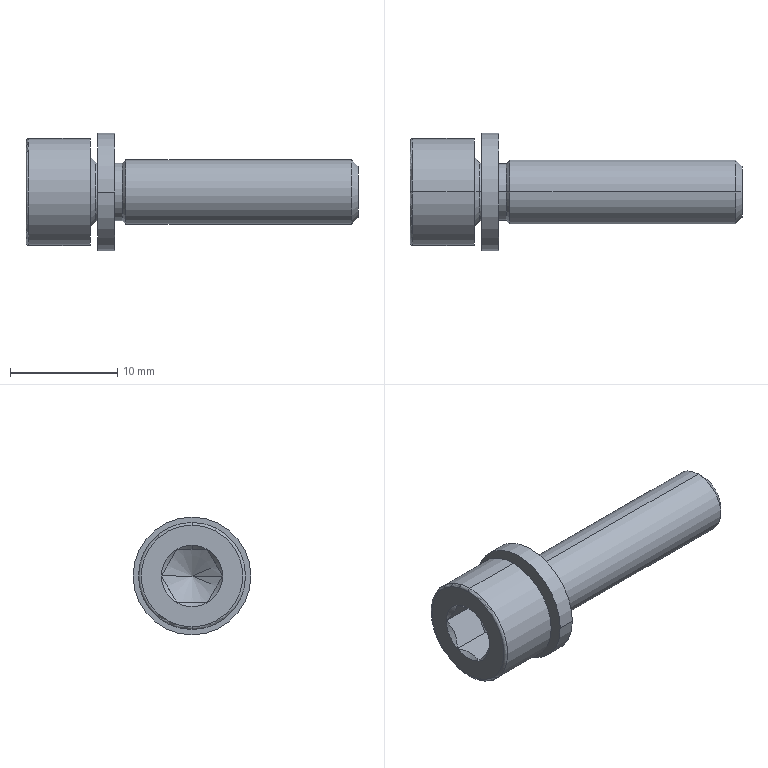Part | SolidWorks | features RevCut 2, Revolution 2, Chamfer 1, Cut 1, Fillet 1 | 2 solids | 48 faces | box 31 x 11 x 11 mm | volume 1178 mm3 | plane 17 | cone 15 | cylinder 10 | torus 6 | commonest cylinder face diameters 5.35 x2 5.62 x2 6 x2 10 x2 11 x2
STEP:
#1=CARTESIAN_POINT('',(8.28,-5.5,0.));
#2=VERTEX_POINT('',#1);
#3=CARTESIAN_POINT('',(8.28,5.5,0.));
#4=VERTEX_POINT('',#3);
#5=CARTESIAN_POINT('',(8.28,0.,0.));
#6=DIRECTION('',(-1.,0.,0.));
#7=DIRECTION('',(0.,-1.,0.));
#8=AXIS2_PLACEMENT_3D('',#5,#6,#7);
#9=CIRCLE('',#8,5.5);
#10=EDGE_CURVE('',#2,#4,#9,.T.);
#11=ORIENTED_EDGE('',*,*,#10,.T.);
#12=CARTESIAN_POINT('',(6.68,5.5,0.));
#13=VERTEX_POINT('',#12);
#14=CARTESIAN_POINT('',(0.,5.5,0.));
#15=DIRECTION('',(-1.,0.,0.));
#16=VECTOR('',#15,1000.);
#17=LINE('',#14,#16);
#18=EDGE_CURVE('',#4,#13,#17,.T.);
#19=ORIENTED_EDGE('',*,*,#18,.T.);
#20=CARTESIAN_POINT('',(6.68,-5.5,0.));
#21=VERTEX_POINT('',#20);
#22=CARTESIAN_POINT('',(6.68,0.,0.));
#23=DIRECTION('',(-1.,0.,0.));
#24=DIRECTION('',(0.,-1.,0.));
#25=AXIS2_PLACEMENT_3D('',#22,#23,#24);
#26=CIRCLE('',#25,5.5);
#27=EDGE_CURVE('',#21,#13,#26,.T.);
#28=ORIENTED_EDGE('',*,*,#27,.F.);
#29=CARTESIAN_POINT('',(0.,-5.5,0.));
#30=DIRECTION('',(-1.,0.,0.));
#31=VECTOR('',#30,1000.);
#32=LINE('',#29,#31);
#33=EDGE_CURVE('',#2,#21,#32,.T.);
#34=ORIENTED_EDGE('',*,*,#33,.F.);
#35=EDGE_LOOP('',(#11,#19,#28,#34));
#36=FACE_OUTER_BOUND('',#35,.T.);
#37=CARTESIAN_POINT('',(0.,0.,0.));
#38=DIRECTION('',(-1.,0.,0.));
#39=DIRECTION('',(0.,-1.,0.));
#40=AXIS2_PLACEMENT_3D('',#37,#38,#39);
#41=CYLINDRICAL_SURFACE('',#40,5.5);
#42=ADVANCED_FACE('',(#36),#41,.T.);
#43=CARTESIAN_POINT('',(8.28,2.81,0.));
#44=VERTEX_POINT('',#43);
#45=CARTESIAN_POINT('',(8.28,-2.81,0.));
#46=VERTEX_POINT('',#45);
#47=CARTESIAN_POINT('',(8.28,0.,0.));
#48=DIRECTION('',(-1.,0.,0.));
#49=DIRECTION('',(0.,-1.,0.));
#50=AXIS2_PLACEMENT_3D('',#47,#48,#49);
#51=CIRCLE('',#50,2.81);
#52=EDGE_CURVE('',#44,#46,#51,.T.);
#53=ORIENTED_EDGE('',*,*,#52,.F.);
#54=CARTESIAN_POINT('',(6.68,2.81,0.));
#55=VERTEX_POINT('',#54);
#56=CARTESIAN_POINT('',(0.,2.81,0.));
#57=DIRECTION('',(-1.,0.,0.));
#58=VECTOR('',#57,1000.);
#59=LINE('',#56,#58);
#60=EDGE_CURVE('',#44,#55,#59,.T.);
#61=ORIENTED_EDGE('',*,*,#60,.T.);
#62=CARTESIAN_POINT('',(6.68,-2.81,0.));
#63=VERTEX_POINT('',#62);
#64=CARTESIAN_POINT('',(6.68,0.,0.));
#65=DIRECTION('',(-1.,0.,0.));
#66=DIRECTION('',(0.,-1.,0.));
#67=AXIS2_PLACEMENT_3D('',#64,#65,#66);
#68=CIRCLE('',#67,2.81);
#69=EDGE_CURVE('',#55,#63,#68,.T.);
#70=ORIENTED_EDGE('',*,*,#69,.T.);
#71=CARTESIAN_POINT('',(0.,-2.81,0.));
#72=DIRECTION('',(-1.,0.,0.));
#73=VECTOR('',#72,1000.);
#74=LINE('',#71,#73);
#75=EDGE_CURVE('',#46,#63,#74,.T.);
#76=ORIENTED_EDGE('',*,*,#75,.F.);
#77=EDGE_LOOP('',(#53,#61,#70,#76));
#78=FACE_OUTER_BOUND('',#77,.T.);
#79=CARTESIAN_POINT('',(0.,0.,0.));
#80=DIRECTION('',(-1.,0.,0.));
#81=DIRECTION('',(0.,-1.,0.));
#82=AXIS2_PLACEMENT_3D('',#79,#80,#81);
#83=CYLINDRICAL_SURFACE('',#82,2.81);
#84=ADVANCED_FACE('',(#78),#83,.F.);
#85=ORIENTED_EDGE('',*,*,#60,.F.);
#86=CARTESIAN_POINT('',(8.28,0.,0.));
#87=DIRECTION('',(-1.,0.,0.));
#88=DIRECTION('',(0.,-1.,0.));
#89=AXIS2_PLACEMENT_3D('',#86,#87,#88);
#90=CIRCLE('',#89,2.81);
#91=EDGE_CURVE('',#46,#44,#90,.T.);
#92=ORIENTED_EDGE('',*,*,#91,.F.);
#93=ORIENTED_EDGE('',*,*,#75,.T.);
#94=CARTESIAN_POINT('',(6.68,0.,0.));
#95=DIRECTION('',(-1.,0.,0.));
#96=DIRECTION('',(0.,-1.,0.));
#97=AXIS2_PLACEMENT_3D('',#94,#95,#96);
#98=CIRCLE('',#97,2.81);
#99=EDGE_CURVE('',#63,#55,#98,.T.);
#100=ORIENTED_EDGE('',*,*,#99,.T.);
#101=EDGE_LOOP('',(#85,#92,#93,#100));
#102=FACE_OUTER_BOUND('',#101,.T.);
#103=CARTESIAN_POINT('',(0.,0.,0.));
#104=DIRECTION('',(-1.,0.,0.));
#105=DIRECTION('',(0.,-1.,0.));
#106=AXIS2_PLACEMENT_3D('',#103,#104,#105);
#107=CYLINDRICAL_SURFACE('',#106,2.81);
#108=ADVANCED_FACE('',(#102),#107,.F.);
#109=ORIENTED_EDGE('',*,*,#99,.F.);
#110=ORIENTED_EDGE('',*,*,#69,.F.);
#111=EDGE_LOOP('',(#109,#110));
#112=FACE_BOUND('',#111,.T.);
#113=ORIENTED_EDGE('',*,*,#27,.T.);
#114=CARTESIAN_POINT('',(6.68,0.,0.));
#115=DIRECTION('',(-1.,0.,0.));
#116=DIRECTION('',(0.,-1.,0.));
#117=AXIS2_PLACEMENT_3D('',#114,#115,#116);
#118=CIRCLE('',#117,5.5);
#119=EDGE_CURVE('',#13,#21,#118,.T.);
#120=ORIENTED_EDGE('',*,*,#119,.T.);
#121=EDGE_LOOP('',(#113,#120));
#122=FACE_OUTER_BOUND('',#121,.T.);
#123=CARTESIAN_POINT('',(6.68,-2.81,0.));
#124=DIRECTION('',(1.,0.,0.));
#125=DIRECTION('',(0.,1.,0.));
#126=AXIS2_PLACEMENT_3D('',#123,#124,#125);
#127=PLANE('',#126);
#128=ADVANCED_FACE('',(#112,#122),#127,.F.);
#129=ORIENTED_EDGE('',*,*,#18,.F.);
#130=CARTESIAN_POINT('',(8.28,0.,0.));
#131=DIRECTION('',(-1.,0.,0.));
#132=DIRECTION('',(0.,-1.,0.));
#133=AXIS2_PLACEMENT_3D('',#130,#131,#132);
#134=CIRCLE('',#133,5.5);
#135=EDGE_CURVE('',#4,#2,#134,.T.);
#136=ORIENTED_EDGE('',*,*,#135,.T.);
#137=ORIENTED_EDGE('',*,*,#33,.T.);
#138=ORIENTED_EDGE('',*,*,#119,.F.);
#139=EDGE_LOOP('',(#129,#136,#137,#138));
#140=FACE_OUTER_BOUND('',#139,.T.);
#141=CARTESIAN_POINT('',(0.,0.,0.));
#142=DIRECTION('',(-1.,0.,0.));
#143=DIRECTION('',(0.,-1.,0.));
#144=AXIS2_PLACEMENT_3D('',#141,#142,#143);
#145=CYLINDRICAL_SURFACE('',#144,5.5);
#146=ADVANCED_FACE('',(#140),#145,.T.);
#147=ORIENTED_EDGE('',*,*,#10,.F.);
#148=ORIENTED_EDGE('',*,*,#135,.F.);
#149=EDGE_LOOP('',(#147,#148));
#150=FACE_OUTER_BOUND('',#149,.T.);
#151=ORIENTED_EDGE('',*,*,#91,.T.);
#152=ORIENTED_EDGE('',*,*,#52,.T.);
#153=EDGE_LOOP('',(#151,#152));
#154=FACE_BOUND('',#153,.T.);
#155=CARTESIAN_POINT('',(8.28,-5.5,0.));
#156=DIRECTION('',(-1.,0.,0.));
#157=DIRECTION('',(0.,-1.,0.));
#158=AXIS2_PLACEMENT_3D('',#155,#156,#157);
#159=PLANE('',#158);
#160=ADVANCED_FACE('',(#150,#154),#159,.F.);
#161=CLOSED_SHELL('',(#42,#84,#108,#128,#146,#160));
#162=MANIFOLD_SOLID_BREP('',#161);
#163=CARTESIAN_POINT('',(31.,0.,-2.4));
#164=VERTEX_POINT('',#163);
#165=CARTESIAN_POINT('',(31.,0.,2.4));
#166=VERTEX_POINT('',#165);
#167=CARTESIAN_POINT('',(31.,0.,0.));
#168=DIRECTION('',(1.,0.,0.));
#169=DIRECTION('',(0.,0.,-1.));
#170=AXIS2_PLACEMENT_3D('',#167,#168,#169);
#171=CIRCLE('',#170,2.4);
#172=EDGE_CURVE('',#164,#166,#171,.T.);
#173=ORIENTED_EDGE('',*,*,#172,.F.);
#174=CARTESIAN_POINT('',(30.4,0.,-3.));
#175=VERTEX_POINT('',#174);
#176=CARTESIAN_POINT('',(31.,0.,-2.4));
#177=DIRECTION('',(-0.7071,0.,-0.7071));
#178=VECTOR('',#177,1000.);
#179=LINE('',#176,#178);
#180=EDGE_CURVE('',#164,#175,#179,.T.);
#181=ORIENTED_EDGE('',*,*,#180,.T.);
#182=CARTESIAN_POINT('',(30.4,0.,3.));
#183=VERTEX_POINT('',#182);
#184=CARTESIAN_POINT('',(30.4,0.,0.));
#185=DIRECTION('',(-1.,0.,0.));
#186=DIRECTION('',(0.,0.,-1.));
#187=AXIS2_PLACEMENT_3D('',#184,#185,#186);
#188=CIRCLE('',#187,3.);
#189=EDGE_CURVE('',#183,#175,#188,.T.);
#190=ORIENTED_EDGE('',*,*,#189,.F.);
#191=CARTESIAN_POINT('',(31.,0.,2.4));
#192=DIRECTION('',(-0.7071,0.,0.7071));
#193=VECTOR('',#192,1000.);
#194=LINE('',#191,#193);
#195=EDGE_CURVE('',#166,#183,#194,.T.);
#196=ORIENTED_EDGE('',*,*,#195,.F.);
#197=EDGE_LOOP('',(#173,#181,#190,#196));
#198=FACE_OUTER_BOUND('',#197,.T.);
#199=CARTESIAN_POINT('',(31.,0.,0.));
#200=DIRECTION('',(-1.,0.,0.));
#201=DIRECTION('',(0.,0.,1.));
#202=AXIS2_PLACEMENT_3D('',#199,#200,#201);
#203=CONICAL_SURFACE('',#202,2.4,0.7854);
#204=ADVANCED_FACE('',(#198),#203,.T.);
#205=CARTESIAN_POINT('',(0.25,0.,-5.));
#206=VERTEX_POINT('',#205);
#207=CARTESIAN_POINT('',(0.25,0.,5.));
#208=VERTEX_POINT('',#207);
#209=CARTESIAN_POINT('',(0.25,0.,0.));
#210=DIRECTION('',(1.,0.,0.));
#211=DIRECTION('',(0.,0.,1.));
#212=AXIS2_PLACEMENT_3D('',#209,#210,#211);
#213=CIRCLE('',#212,5.);
#214=EDGE_CURVE('',#206,#208,#213,.T.);
#215=ORIENTED_EDGE('',*,*,#214,.F.);
#216=CARTESIAN_POINT('',(0.,0.,-4.75));
#217=VERTEX_POINT('',#216);
#218=CARTESIAN_POINT('',(0.25,0.,-4.75));
#219=DIRECTION('',(0.,1.,0.));
#220=DIRECTION('',(0.,0.,1.));
#221=AXIS2_PLACEMENT_3D('',#218,#219,#220);
#222=CIRCLE('',#221,0.25);
#223=EDGE_CURVE('',#206,#217,#222,.T.);
#224=ORIENTED_EDGE('',*,*,#223,.T.);
#225=CARTESIAN_POINT('',(0.,0.,4.75));
#226=VERTEX_POINT('',#225);
#227=CARTESIAN_POINT('',(0.,0.,0.));
#228=DIRECTION('',(-1.,0.,0.));
#229=DIRECTION('',(0.,0.,1.));
#230=AXIS2_PLACEMENT_3D('',#227,#228,#229);
#231=CIRCLE('',#230,4.75);
#232=EDGE_CURVE('',#226,#217,#231,.T.);
#233=ORIENTED_EDGE('',*,*,#232,.F.);
#234=CARTESIAN_POINT('',(0.25,0.,4.75));
#235=DIRECTION('',(0.,-1.,0.));
#236=DIRECTION('',(0.,0.,-1.));
#237=AXIS2_PLACEMENT_3D('',#234,#235,#236);
#238=CIRCLE('',#237,0.25);
#239=EDGE_CURVE('',#208,#226,#238,.T.);
#240=ORIENTED_EDGE('',*,*,#239,.F.);
#241=EDGE_LOOP('',(#215,#224,#233,#240));
#242=FACE_OUTER_BOUND('',#241,.T.);
#243=CARTESIAN_POINT('',(0.25,0.,0.));
#244=DIRECTION('',(-1.,0.,0.));
#245=DIRECTION('',(0.,0.,1.));
#246=AXIS2_PLACEMENT_3D('',#243,#244,#245);
#247=TOROIDAL_SURFACE('',#246,4.75,0.25);
#248=ADVANCED_FACE('',(#242),#247,.T.);
#249=CARTESIAN_POINT('',(5.351,0.,0.));
#250=VERTEX_POINT('',#249);
#251=CARTESIAN_POINT('',(3.7,-2.86,0.));
#252=VERTEX_POINT('',#251);
#253=CARTESIAN_POINT('',(5.351,0.,0.));
#254=DIRECTION('',(-0.5,-0.866,0.));
#255=VECTOR('',#254,1000.);
#256=LINE('',#253,#255);
#257=EDGE_CURVE('',#250,#252,#256,.T.);
#258=ORIENTED_EDGE('',*,*,#257,.F.);
#259=CARTESIAN_POINT('',(3.7,2.86,0.));
#260=VERTEX_POINT('',#259);
#261=CARTESIAN_POINT('',(5.351,0.,0.));
#262=DIRECTION('',(-0.5,0.866,0.));
#263=VECTOR('',#262,1000.);
#264=LINE('',#261,#263);
#265=EDGE_CURVE('',#250,#260,#264,.T.);
#266=ORIENTED_EDGE('',*,*,#265,.T.);
#267=CARTESIAN_POINT('',(3.7,1.43,-2.477));
#268=VERTEX_POINT('',#267);
#269=CARTESIAN_POINT('',(3.7,0.,0.));
#270=DIRECTION('',(-1.,0.,0.));
#271=DIRECTION('',(0.,-1.,0.));
#272=AXIS2_PLACEMENT_3D('',#269,#270,#271);
#273=CIRCLE('',#272,2.86);
#274=EDGE_CURVE('',#260,#268,#273,.T.);
#275=ORIENTED_EDGE('',*,*,#274,.T.);
#276=CARTESIAN_POINT('',(3.7,-1.43,-2.477));
#277=VERTEX_POINT('',#276);
#278=CARTESIAN_POINT('',(3.7,0.,0.));
#279=DIRECTION('',(-1.,0.,0.));
#280=DIRECTION('',(0.,-1.,0.));
#281=AXIS2_PLACEMENT_3D('',#278,#279,#280);
#282=CIRCLE('',#281,2.86);
#283=EDGE_CURVE('',#268,#277,#282,.T.);
#284=ORIENTED_EDGE('',*,*,#283,.T.);
#285=CARTESIAN_POINT('',(3.7,0.,0.));
#286=DIRECTION('',(-1.,0.,0.));
#287=DIRECTION('',(0.,-1.,0.));
#288=AXIS2_PLACEMENT_3D('',#285,#286,#287);
#289=CIRCLE('',#288,2.86);
#290=EDGE_CURVE('',#277,#252,#289,.T.);
#291=ORIENTED_EDGE('',*,*,#290,.T.);
#292=EDGE_LOOP('',(#258,#266,#275,#284,#291));
#293=FACE_OUTER_BOUND('',#292,.T.);
#294=CARTESIAN_POINT('',(-994.649,0.,0.));
#295=DIRECTION('',(-1.,0.,0.));
#296=DIRECTION('',(0.,-1.,0.));
#297=AXIS2_PLACEMENT_3D('',#294,#295,#296);
#298=CONICAL_SURFACE('',#297,1732.051,1.047);
#299=ADVANCED_FACE('',(#293),#298,.F.);
#300=CARTESIAN_POINT('',(0.3832,0.,2.477));
#301=VERTEX_POINT('',#300);
#302=CARTESIAN_POINT('',(0.,1.43,2.477));
#303=VERTEX_POINT('',#302);
#304=CARTESIAN_POINT('',(0.3832,0.,2.477));
#305=CARTESIAN_POINT('',(0.3832,0.2515,2.477));
#306=CARTESIAN_POINT('',(0.3444,0.4963,2.477));
#307=CARTESIAN_POINT('',(0.2078,0.9759,2.477));
#308=CARTESIAN_POINT('',(0.1107,1.209,2.477));
#309=CARTESIAN_POINT('',(0.,1.43,2.477));
#310=B_SPLINE_CURVE_WITH_KNOTS('',3,(#304,#305,#306,#307,#308,#309),.UNSPECIFIED.,.F.,.F.,(4,2,4),(0.003339,0.004081,0.004823),.UNSPECIFIED.);
#311=EDGE_CURVE('',#301,#303,#310,.T.);
#312=ORIENTED_EDGE('',*,*,#311,.F.);
#313=CARTESIAN_POINT('',(0.,0.,2.86));
#314=VERTEX_POINT('',#313);
#315=CARTESIAN_POINT('',(0.3832,0.,2.477));
#316=DIRECTION('',(-0.7071,0.,0.7071));
#317=VECTOR('',#316,1000.);
#318=LINE('',#315,#317);
#319=EDGE_CURVE('',#301,#314,#318,.T.);
#320=ORIENTED_EDGE('',*,*,#319,.T.);
#321=CARTESIAN_POINT('',(0.,0.,0.));
#322=DIRECTION('',(1.,0.,0.));
#323=DIRECTION('',(0.,0.,-1.));
#324=AXIS2_PLACEMENT_3D('',#321,#322,#323);
#325=CIRCLE('',#324,2.86);
#326=EDGE_CURVE('',#303,#314,#325,.T.);
#327=ORIENTED_EDGE('',*,*,#326,.F.);
#328=EDGE_LOOP('',(#312,#320,#327));
#329=FACE_OUTER_BOUND('',#328,.T.);
#330=CARTESIAN_POINT('',(0.3832,0.,0.));
#331=DIRECTION('',(-1.,0.,0.));
#332=DIRECTION('',(0.,0.,1.));
#333=AXIS2_PLACEMENT_3D('',#330,#331,#332);
#334=CONICAL_SURFACE('',#333,2.477,0.7854);
#335=ADVANCED_FACE('',(#329),#334,.F.);
#336=CARTESIAN_POINT('',(9.325,0.,-3.));
#337=VERTEX_POINT('',#336);
#338=CARTESIAN_POINT('',(9.325,0.,3.));
#339=VERTEX_POINT('',#338);
#340=CARTESIAN_POINT('',(9.325,0.,0.));
#341=DIRECTION('',(1.,0.,0.));
#342=DIRECTION('',(0.,0.,-1.));
#343=AXIS2_PLACEMENT_3D('',#340,#341,#342);
#344=CIRCLE('',#343,3.);
#345=EDGE_CURVE('',#337,#339,#344,.T.);
#346=ORIENTED_EDGE('',*,*,#345,.T.);
#347=CARTESIAN_POINT('',(0.,0.,3.));
#348=DIRECTION('',(1.,0.,0.));
#349=VECTOR('',#348,1000.);
#350=LINE('',#347,#349);
#351=EDGE_CURVE('',#339,#183,#350,.T.);
#352=ORIENTED_EDGE('',*,*,#351,.T.);
#353=ORIENTED_EDGE('',*,*,#189,.T.);
#354=CARTESIAN_POINT('',(0.,0.,-3.));
#355=DIRECTION('',(1.,0.,0.));
#356=VECTOR('',#355,1000.);
#357=LINE('',#354,#356);
#358=EDGE_CURVE('',#337,#175,#357,.T.);
#359=ORIENTED_EDGE('',*,*,#358,.F.);
#360=EDGE_LOOP('',(#346,#352,#353,#359));
#361=FACE_OUTER_BOUND('',#360,.T.);
#362=CARTESIAN_POINT('',(0.,0.,0.));
#363=DIRECTION('',(1.,0.,0.));
#364=DIRECTION('',(0.,0.,-1.));
#365=AXIS2_PLACEMENT_3D('',#362,#363,#364);
#366=CYLINDRICAL_SURFACE('',#365,3.);
#367=ADVANCED_FACE('',(#361),#366,.T.);
#368=CARTESIAN_POINT('',(9.,0.,-2.675));
#369=VERTEX_POINT('',#368);
#370=CARTESIAN_POINT('',(9.,0.,2.675));
#371=VERTEX_POINT('',#370);
#372=CARTESIAN_POINT('',(9.,0.,0.));
#373=DIRECTION('',(1.,0.,0.));
#374=DIRECTION('',(0.,0.,-1.));
#375=AXIS2_PLACEMENT_3D('',#372,#373,#374);
#376=CIRCLE('',#375,2.675);
#377=EDGE_CURVE('',#369,#371,#376,.T.);
#378=ORIENTED_EDGE('',*,*,#377,.T.);
#379=CARTESIAN_POINT('',(9.325,0.,3.));
#380=DIRECTION('',(0.7071,0.,0.7071));
#381=VECTOR('',#380,1000.);
#382=LINE('',#379,#381);
#383=EDGE_CURVE('',#371,#339,#382,.T.);
#384=ORIENTED_EDGE('',*,*,#383,.T.);
#385=ORIENTED_EDGE('',*,*,#345,.F.);
#386=CARTESIAN_POINT('',(9.325,0.,-3.));
#387=DIRECTION('',(0.7071,0.,-0.7071));
#388=VECTOR('',#387,1000.);
#389=LINE('',#386,#388);
#390=EDGE_CURVE('',#369,#337,#389,.T.);
#391=ORIENTED_EDGE('',*,*,#390,.F.);
#392=EDGE_LOOP('',(#378,#384,#385,#391));
#393=FACE_OUTER_BOUND('',#392,.T.);
#394=CARTESIAN_POINT('',(9.325,0.,0.));
#395=DIRECTION('',(1.,0.,0.));
#396=DIRECTION('',(0.,0.,-1.));
#397=AXIS2_PLACEMENT_3D('',#394,#395,#396);
#398=CONICAL_SURFACE('',#397,3.,0.7854);
#399=ADVANCED_FACE('',(#393),#398,.T.);
#400=CARTESIAN_POINT('',(6.68,0.,-2.675));
#401=VERTEX_POINT('',#400);
#402=CARTESIAN_POINT('',(6.68,0.,2.675));
#403=VERTEX_POINT('',#402);
#404=CARTESIAN_POINT('',(6.68,0.,0.));
#405=DIRECTION('',(1.,0.,0.));
#406=DIRECTION('',(0.,0.,-1.));
#407=AXIS2_PLACEMENT_3D('',#404,#405,#406);
#408=CIRCLE('',#407,2.675);
#409=EDGE_CURVE('',#401,#403,#408,.T.);
#410=ORIENTED_EDGE('',*,*,#409,.T.);
#411=CARTESIAN_POINT('',(0.,0.,2.675));
#412=DIRECTION('',(1.,0.,0.));
#413=VECTOR('',#412,1000.);
#414=LINE('',#411,#413);
#415=EDGE_CURVE('',#403,#371,#414,.T.);
#416=ORIENTED_EDGE('',*,*,#415,.T.);
#417=ORIENTED_EDGE('',*,*,#377,.F.);
#418=CARTESIAN_POINT('',(0.,0.,-2.675));
#419=DIRECTION('',(1.,0.,0.));
#420=VECTOR('',#419,1000.);
#421=LINE('',#418,#420);
#422=EDGE_CURVE('',#401,#369,#421,.T.);
#423=ORIENTED_EDGE('',*,*,#422,.F.);
#424=EDGE_LOOP('',(#410,#416,#417,#423));
#425=FACE_OUTER_BOUND('',#424,.T.);
#426=CARTESIAN_POINT('',(0.,0.,0.));
#427=DIRECTION('',(1.,0.,0.));
#428=DIRECTION('',(0.,0.,-1.));
#429=AXIS2_PLACEMENT_3D('',#426,#427,#428);
#430=CYLINDRICAL_SURFACE('',#429,2.675);
#431=ADVANCED_FACE('',(#425),#430,.T.);
#432=CARTESIAN_POINT('',(6.68,0.,0.));
#433=DIRECTION('',(1.,0.,0.));
#434=DIRECTION('',(0.,0.,-1.));
#435=AXIS2_PLACEMENT_3D('',#432,#433,#434);
#436=CIRCLE('',#435,2.675);
#437=EDGE_CURVE('',#403,#401,#436,.T.);
#438=ORIENTED_EDGE('',*,*,#437,.F.);
#439=CARTESIAN_POINT('',(6.495,0.,2.757));
#440=VERTEX_POINT('',#439);
#441=CARTESIAN_POINT('',(6.68,0.,2.925));
#442=DIRECTION('',(0.,1.,0.));
#443=DIRECTION('',(0.,0.,1.));
#444=AXIS2_PLACEMENT_3D('',#441,#442,#443);
#445=CIRCLE('',#444,0.25);
#446=EDGE_CURVE('',#403,#440,#445,.T.);
#447=ORIENTED_EDGE('',*,*,#446,.T.);
#448=CARTESIAN_POINT('',(6.495,0.,-2.757));
#449=VERTEX_POINT('',#448);
#450=CARTESIAN_POINT('',(6.495,0.,0.));
#451=DIRECTION('',(1.,0.,0.));
#452=DIRECTION('',(0.,0.,-1.));
#453=AXIS2_PLACEMENT_3D('',#450,#451,#452);
#454=CIRCLE('',#453,2.757);
#455=EDGE_CURVE('',#440,#449,#454,.T.);
#456=ORIENTED_EDGE('',*,*,#455,.T.);
#457=CARTESIAN_POINT('',(6.68,0.,-2.925));
#458=DIRECTION('',(0.,-1.,0.));
#459=DIRECTION('',(0.,0.,-1.));
#460=AXIS2_PLACEMENT_3D('',#457,#458,#459);
#461=CIRCLE('',#460,0.25);
#462=EDGE_CURVE('',#401,#449,#461,.T.);
#463=ORIENTED_EDGE('',*,*,#462,.F.);
#464=EDGE_LOOP('',(#438,#447,#456,#463));
#465=FACE_OUTER_BOUND('',#464,.T.);
#466=CARTESIAN_POINT('',(6.68,0.,0.));
#467=DIRECTION('',(1.,0.,0.));
#468=DIRECTION('',(0.,0.,-1.));
#469=AXIS2_PLACEMENT_3D('',#466,#467,#468);
#470=TOROIDAL_SURFACE('',#469,2.925,0.25);
#471=ADVANCED_FACE('',(#465),#470,.F.);
#472=CARTESIAN_POINT('',(6.495,0.,0.));
#473=DIRECTION('',(1.,0.,0.));
#474=DIRECTION('',(0.,0.,-1.));
#475=AXIS2_PLACEMENT_3D('',#472,#473,#474);
#476=CIRCLE('',#475,2.757);
#477=EDGE_CURVE('',#449,#440,#476,.T.);
#478=ORIENTED_EDGE('',*,*,#477,.F.);
#479=CARTESIAN_POINT('',(6.065,0.,-3.232));
#480=VERTEX_POINT('',#479);
#481=CARTESIAN_POINT('',(6.495,0.,-2.757));
#482=DIRECTION('',(-0.6711,0.,-0.7414));
#483=VECTOR('',#482,1000.);
#484=LINE('',#481,#483);
#485=EDGE_CURVE('',#449,#480,#484,.T.);
#486=ORIENTED_EDGE('',*,*,#485,.T.);
#487=CARTESIAN_POINT('',(6.065,0.,3.232));
#488=VERTEX_POINT('',#487);
#489=CARTESIAN_POINT('',(6.065,0.,0.));
#490=DIRECTION('',(1.,0.,0.));
#491=DIRECTION('',(0.,0.,-1.));
#492=AXIS2_PLACEMENT_3D('',#489,#490,#491);
#493=CIRCLE('',#492,3.232);
#494=EDGE_CURVE('',#480,#488,#493,.T.);
#495=ORIENTED_EDGE('',*,*,#494,.T.);
#496=CARTESIAN_POINT('',(6.495,0.,2.757));
#497=DIRECTION('',(-0.6711,0.,0.7414));
#498=VECTOR('',#497,1000.);
#499=LINE('',#496,#498);
#500=EDGE_CURVE('',#440,#488,#499,.T.);
#501=ORIENTED_EDGE('',*,*,#500,.F.);
#502=EDGE_LOOP('',(#478,#486,#495,#501));
#503=FACE_OUTER_BOUND('',#502,.T.);
#504=CARTESIAN_POINT('',(6.495,0.,0.));
#505=DIRECTION('',(-1.,0.,0.));
#506=DIRECTION('',(0.,0.,1.));
#507=AXIS2_PLACEMENT_3D('',#504,#505,#506);
#508=CONICAL_SURFACE('',#507,2.757,0.8351);
#509=ADVANCED_FACE('',(#503),#508,.T.);
#510=CARTESIAN_POINT('',(6.065,0.,0.));
#511=DIRECTION('',(1.,0.,0.));
#512=DIRECTION('',(0.,0.,-1.));
#513=AXIS2_PLACEMENT_3D('',#510,#511,#512);
#514=CIRCLE('',#513,3.232);
#515=EDGE_CURVE('',#488,#480,#514,.T.);
#516=ORIENTED_EDGE('',*,*,#515,.F.);
#517=CARTESIAN_POINT('',(6.,0.,3.4));
#518=VERTEX_POINT('',#517);
#519=CARTESIAN_POINT('',(6.25,0.,3.4));
#520=DIRECTION('',(0.,1.,0.));
#521=DIRECTION('',(0.,0.,1.));
#522=AXIS2_PLACEMENT_3D('',#519,#520,#521);
#523=CIRCLE('',#522,0.25);
#524=EDGE_CURVE('',#488,#518,#523,.T.);
#525=ORIENTED_EDGE('',*,*,#524,.T.);
#526=CARTESIAN_POINT('',(6.,0.,-3.4));
#527=VERTEX_POINT('',#526);
#528=CARTESIAN_POINT('',(6.,0.,0.));
#529=DIRECTION('',(1.,0.,0.));
#530=DIRECTION('',(0.,0.,-1.));
#531=AXIS2_PLACEMENT_3D('',#528,#529,#530);
#532=CIRCLE('',#531,3.4);
#533=EDGE_CURVE('',#518,#527,#532,.T.);
#534=ORIENTED_EDGE('',*,*,#533,.T.);
#535=CARTESIAN_POINT('',(6.25,0.,-3.4));
#536=DIRECTION('',(0.,-1.,0.));
#537=DIRECTION('',(0.,0.,-1.));
#538=AXIS2_PLACEMENT_3D('',#535,#536,#537);
#539=CIRCLE('',#538,0.25);
#540=EDGE_CURVE('',#480,#527,#539,.T.);
#541=ORIENTED_EDGE('',*,*,#540,.F.);
#542=EDGE_LOOP('',(#516,#525,#534,#541));
#543=FACE_OUTER_BOUND('',#542,.T.);
#544=CARTESIAN_POINT('',(6.25,0.,0.));
#545=DIRECTION('',(1.,0.,0.));
#546=DIRECTION('',(0.,0.,-1.));
#547=AXIS2_PLACEMENT_3D('',#544,#545,#546);
#548=TOROIDAL_SURFACE('',#547,3.4,0.25);
#549=ADVANCED_FACE('',(#543),#548,.F.);
#550=ORIENTED_EDGE('',*,*,#214,.T.);
#551=CARTESIAN_POINT('',(6.,0.,5.));
#552=VERTEX_POINT('',#551);
#553=CARTESIAN_POINT('',(0.,0.,5.));
#554=DIRECTION('',(1.,0.,0.));
#555=VECTOR('',#554,1000.);
#556=LINE('',#553,#555);
#557=EDGE_CURVE('',#208,#552,#556,.T.);
#558=ORIENTED_EDGE('',*,*,#557,.T.);
#559=CARTESIAN_POINT('',(6.,0.,-5.));
#560=VERTEX_POINT('',#559);
#561=CARTESIAN_POINT('',(6.,0.,0.));
#562=DIRECTION('',(1.,0.,0.));
#563=DIRECTION('',(0.,0.,-1.));
#564=AXIS2_PLACEMENT_3D('',#561,#562,#563);
#565=CIRCLE('',#564,5.);
#566=EDGE_CURVE('',#560,#552,#565,.T.);
#567=ORIENTED_EDGE('',*,*,#566,.F.);
#568=CARTESIAN_POINT('',(0.,0.,-5.));
#569=DIRECTION('',(1.,0.,0.));
#570=VECTOR('',#569,1000.);
#571=LINE('',#568,#570);
#572=EDGE_CURVE('',#206,#560,#571,.T.);
#573=ORIENTED_EDGE('',*,*,#572,.F.);
#574=EDGE_LOOP('',(#550,#558,#567,#573));
#575=FACE_OUTER_BOUND('',#574,.T.);
#576=CARTESIAN_POINT('',(0.,0.,0.));
#577=DIRECTION('',(1.,0.,0.));
#578=DIRECTION('',(0.,0.,-1.));
#579=AXIS2_PLACEMENT_3D('',#576,#577,#578);
#580=CYLINDRICAL_SURFACE('',#579,5.);
#581=ADVANCED_FACE('',(#575),#580,.T.);
#582=ORIENTED_EDGE('',*,*,#232,.T.);
#583=CARTESIAN_POINT('',(0.,0.,0.));
#584=DIRECTION('',(-1.,0.,0.));
#585=DIRECTION('',(0.,0.,1.));
#586=AXIS2_PLACEMENT_3D('',#583,#584,#585);
#587=CIRCLE('',#586,4.75);
#588=EDGE_CURVE('',#217,#226,#587,.T.);
#589=ORIENTED_EDGE('',*,*,#588,.T.);
#590=EDGE_LOOP('',(#582,#589));
#591=FACE_OUTER_BOUND('',#590,.T.);
#592=CARTESIAN_POINT('',(0.,2.86,0.));
#593=VERTEX_POINT('',#592);
#594=CARTESIAN_POINT('',(0.,0.,0.));
#595=DIRECTION('',(1.,0.,0.));
#596=DIRECTION('',(0.,0.,-1.));
#597=AXIS2_PLACEMENT_3D('',#594,#595,#596);
#598=CIRCLE('',#597,2.86);
#599=EDGE_CURVE('',#593,#303,#598,.T.);
#600=ORIENTED_EDGE('',*,*,#599,.T.);
#601=ORIENTED_EDGE('',*,*,#326,.T.);
#602=CARTESIAN_POINT('',(0.,-1.43,2.477));
#603=VERTEX_POINT('',#602);
#604=CARTESIAN_POINT('',(0.,0.,0.));
#605=DIRECTION('',(1.,0.,0.));
#606=DIRECTION('',(0.,0.,-1.));
#607=AXIS2_PLACEMENT_3D('',#604,#605,#606);
#608=CIRCLE('',#607,2.86);
#609=EDGE_CURVE('',#314,#603,#608,.T.);
#610=ORIENTED_EDGE('',*,*,#609,.T.);
#611=CARTESIAN_POINT('',(0.,-2.86,0.));
#612=VERTEX_POINT('',#611);
#613=CARTESIAN_POINT('',(0.,0.,0.));
#614=DIRECTION('',(1.,0.,0.));
#615=DIRECTION('',(0.,0.,-1.));
#616=AXIS2_PLACEMENT_3D('',#613,#614,#615);
#617=CIRCLE('',#616,2.86);
#618=EDGE_CURVE('',#603,#612,#617,.T.);
#619=ORIENTED_EDGE('',*,*,#618,.T.);
#620=CARTESIAN_POINT('',(0.,-1.43,-2.477));
#621=VERTEX_POINT('',#620);
#622=CARTESIAN_POINT('',(0.,0.,0.));
#623=DIRECTION('',(1.,0.,0.));
#624=DIRECTION('',(0.,0.,-1.));
#625=AXIS2_PLACEMENT_3D('',#622,#623,#624);
#626=CIRCLE('',#625,2.86);
#627=EDGE_CURVE('',#612,#621,#626,.T.);
#628=ORIENTED_EDGE('',*,*,#627,.T.);
#629=CARTESIAN_POINT('',(0.,1.43,-2.477));
#630=VERTEX_POINT('',#629);
#631=CARTESIAN_POINT('',(0.,0.,0.));
#632=DIRECTION('',(1.,0.,0.));
#633=DIRECTION('',(0.,0.,-1.));
#634=AXIS2_PLACEMENT_3D('',#631,#632,#633);
#635=CIRCLE('',#634,2.86);
#636=EDGE_CURVE('',#621,#630,#635,.T.);
#637=ORIENTED_EDGE('',*,*,#636,.T.);
#638=CARTESIAN_POINT('',(0.,0.,0.));
#639=DIRECTION('',(1.,0.,0.));
#640=DIRECTION('',(0.,0.,-1.));
#641=AXIS2_PLACEMENT_3D('',#638,#639,#640);
#642=CIRCLE('',#641,2.86);
#643=EDGE_CURVE('',#630,#593,#642,.T.);
#644=ORIENTED_EDGE('',*,*,#643,.T.);
#645=EDGE_LOOP('',(#600,#601,#610,#619,#628,#637,#644));
#646=FACE_BOUND('',#645,.T.);
#647=CARTESIAN_POINT('',(0.,0.,0.));
#648=DIRECTION('',(-1.,0.,0.));
#649=DIRECTION('',(0.,0.,1.));
#650=AXIS2_PLACEMENT_3D('',#647,#648,#649);
#651=PLANE('',#650);
#652=ADVANCED_FACE('',(#591,#646),#651,.T.);
#653=ORIENTED_EDGE('',*,*,#557,.F.);
#654=CARTESIAN_POINT('',(0.25,0.,0.));
#655=DIRECTION('',(1.,0.,0.));
#656=DIRECTION('',(0.,0.,1.));
#657=AXIS2_PLACEMENT_3D('',#654,#655,#656);
#658=CIRCLE('',#657,5.);
#659=EDGE_CURVE('',#208,#206,#658,.T.);
#660=ORIENTED_EDGE('',*,*,#659,.T.);
#661=ORIENTED_EDGE('',*,*,#572,.T.);
#662=CARTESIAN_POINT('',(6.,0.,0.));
#663=DIRECTION('',(1.,0.,0.));
#664=DIRECTION('',(0.,0.,-1.));
#665=AXIS2_PLACEMENT_3D('',#662,#663,#664);
#666=CIRCLE('',#665,5.);
#667=EDGE_CURVE('',#552,#560,#666,.T.);
#668=ORIENTED_EDGE('',*,*,#667,.F.);
#669=EDGE_LOOP('',(#653,#660,#661,#668));
#670=FACE_OUTER_BOUND('',#669,.T.);
#671=CARTESIAN_POINT('',(0.,0.,0.));
#672=DIRECTION('',(1.,0.,0.));
#673=DIRECTION('',(0.,0.,-1.));
#674=AXIS2_PLACEMENT_3D('',#671,#672,#673);
#675=CYLINDRICAL_SURFACE('',#674,5.);
#676=ADVANCED_FACE('',(#670),#675,.T.);
#677=ORIENTED_EDGE('',*,*,#566,.T.);
#678=ORIENTED_EDGE('',*,*,#667,.T.);
#679=EDGE_LOOP('',(#677,#678));
#680=FACE_OUTER_BOUND('',#679,.T.);
#681=CARTESIAN_POINT('',(6.,0.,0.));
#682=DIRECTION('',(1.,0.,0.));
#683=DIRECTION('',(0.,0.,-1.));
#684=AXIS2_PLACEMENT_3D('',#681,#682,#683);
#685=CIRCLE('',#684,3.4);
#686=EDGE_CURVE('',#527,#518,#685,.T.);
#687=ORIENTED_EDGE('',*,*,#686,.F.);
#688=ORIENTED_EDGE('',*,*,#533,.F.);
#689=EDGE_LOOP('',(#687,#688));
#690=FACE_BOUND('',#689,.T.);
#691=CARTESIAN_POINT('',(6.,5.,0.));
#692=DIRECTION('',(1.,0.,0.));
#693=DIRECTION('',(0.,0.,-1.));
#694=AXIS2_PLACEMENT_3D('',#691,#692,#693);
#695=PLANE('',#694);
#696=ADVANCED_FACE('',(#680,#690),#695,.T.);
#697=ORIENTED_EDGE('',*,*,#524,.F.);
#698=ORIENTED_EDGE('',*,*,#494,.F.);
#699=ORIENTED_EDGE('',*,*,#540,.T.);
#700=ORIENTED_EDGE('',*,*,#686,.T.);
#701=EDGE_LOOP('',(#697,#698,#699,#700));
#702=FACE_OUTER_BOUND('',#701,.T.);
#703=CARTESIAN_POINT('',(6.25,0.,0.));
#704=DIRECTION('',(1.,0.,0.));
#705=DIRECTION('',(0.,0.,-1.));
#706=AXIS2_PLACEMENT_3D('',#703,#704,#705);
#707=TOROIDAL_SURFACE('',#706,3.4,0.25);
#708=ADVANCED_FACE('',(#702),#707,.F.);
#709=ORIENTED_EDGE('',*,*,#485,.F.);
#710=ORIENTED_EDGE('',*,*,#455,.F.);
#711=ORIENTED_EDGE('',*,*,#500,.T.);
#712=ORIENTED_EDGE('',*,*,#515,.T.);
#713=EDGE_LOOP('',(#709,#710,#711,#712));
#714=FACE_OUTER_BOUND('',#713,.T.);
#715=CARTESIAN_POINT('',(6.495,0.,0.));
#716=DIRECTION('',(-1.,0.,0.));
#717=DIRECTION('',(0.,0.,1.));
#718=AXIS2_PLACEMENT_3D('',#715,#716,#717);
#719=CONICAL_SURFACE('',#718,2.757,0.8351);
#720=ADVANCED_FACE('',(#714),#719,.T.);
#721=ORIENTED_EDGE('',*,*,#446,.F.);
#722=ORIENTED_EDGE('',*,*,#409,.F.);
#723=ORIENTED_EDGE('',*,*,#462,.T.);
#724=ORIENTED_EDGE('',*,*,#477,.T.);
#725=EDGE_LOOP('',(#721,#722,#723,#724));
#726=FACE_OUTER_BOUND('',#725,.T.);
#727=CARTESIAN_POINT('',(6.68,0.,0.));
#728=DIRECTION('',(1.,0.,0.));
#729=DIRECTION('',(0.,0.,-1.));
#730=AXIS2_PLACEMENT_3D('',#727,#728,#729);
#731=TOROIDAL_SURFACE('',#730,2.925,0.25);
#732=ADVANCED_FACE('',(#726),#731,.F.);
#733=ORIENTED_EDGE('',*,*,#415,.F.);
#734=ORIENTED_EDGE('',*,*,#437,.T.);
#735=ORIENTED_EDGE('',*,*,#422,.T.);
#736=CARTESIAN_POINT('',(9.,0.,0.));
#737=DIRECTION('',(1.,0.,0.));
#738=DIRECTION('',(0.,0.,-1.));
#739=AXIS2_PLACEMENT_3D('',#736,#737,#738);
#740=CIRCLE('',#739,2.675);
#741=EDGE_CURVE('',#371,#369,#740,.T.);
#742=ORIENTED_EDGE('',*,*,#741,.F.);
#743=EDGE_LOOP('',(#733,#734,#735,#742));
#744=FACE_OUTER_BOUND('',#743,.T.);
#745=CARTESIAN_POINT('',(0.,0.,0.));
#746=DIRECTION('',(1.,0.,0.));
#747=DIRECTION('',(0.,0.,-1.));
#748=AXIS2_PLACEMENT_3D('',#745,#746,#747);
#749=CYLINDRICAL_SURFACE('',#748,2.675);
#750=ADVANCED_FACE('',(#744),#749,.T.);
#751=ORIENTED_EDGE('',*,*,#383,.F.);
#752=ORIENTED_EDGE('',*,*,#741,.T.);
#753=ORIENTED_EDGE('',*,*,#390,.T.);
#754=CARTESIAN_POINT('',(9.325,0.,0.));
#755=DIRECTION('',(1.,0.,0.));
#756=DIRECTION('',(0.,0.,-1.));
#757=AXIS2_PLACEMENT_3D('',#754,#755,#756);
#758=CIRCLE('',#757,3.);
#759=EDGE_CURVE('',#339,#337,#758,.T.);
#760=ORIENTED_EDGE('',*,*,#759,.F.);
#761=EDGE_LOOP('',(#751,#752,#753,#760));
#762=FACE_OUTER_BOUND('',#761,.T.);
#763=CARTESIAN_POINT('',(9.325,0.,0.));
#764=DIRECTION('',(1.,0.,0.));
#765=DIRECTION('',(0.,0.,-1.));
#766=AXIS2_PLACEMENT_3D('',#763,#764,#765);
#767=CONICAL_SURFACE('',#766,3.,0.7854);
#768=ADVANCED_FACE('',(#762),#767,.T.);
#769=ORIENTED_EDGE('',*,*,#351,.F.);
#770=ORIENTED_EDGE('',*,*,#759,.T.);
#771=ORIENTED_EDGE('',*,*,#358,.T.);
#772=CARTESIAN_POINT('',(30.4,0.,0.));
#773=DIRECTION('',(-1.,0.,0.));
#774=DIRECTION('',(0.,0.,-1.));
#775=AXIS2_PLACEMENT_3D('',#772,#773,#774);
#776=CIRCLE('',#775,3.);
#777=EDGE_CURVE('',#175,#183,#776,.T.);
#778=ORIENTED_EDGE('',*,*,#777,.T.);
#779=EDGE_LOOP('',(#769,#770,#771,#778));
#780=FACE_OUTER_BOUND('',#779,.T.);
#781=CARTESIAN_POINT('',(0.,0.,0.));
#782=DIRECTION('',(1.,0.,0.));
#783=DIRECTION('',(0.,0.,-1.));
#784=AXIS2_PLACEMENT_3D('',#781,#782,#783);
#785=CYLINDRICAL_SURFACE('',#784,3.);
#786=ADVANCED_FACE('',(#780),#785,.T.);
#787=CARTESIAN_POINT('',(31.,0.,0.));
#788=DIRECTION('',(1.,0.,0.));
#789=DIRECTION('',(0.,0.,-1.));
#790=AXIS2_PLACEMENT_3D('',#787,#788,#789);
#791=CIRCLE('',#790,2.4);
#792=EDGE_CURVE('',#166,#164,#791,.T.);
#793=ORIENTED_EDGE('',*,*,#792,.T.);
#794=ORIENTED_EDGE('',*,*,#172,.T.);
#795=EDGE_LOOP('',(#793,#794));
#796=FACE_OUTER_BOUND('',#795,.T.);
#797=CARTESIAN_POINT('',(31.,3.,0.));
#798=DIRECTION('',(1.,0.,0.));
#799=DIRECTION('',(0.,0.,-1.));
#800=AXIS2_PLACEMENT_3D('',#797,#798,#799);
#801=PLANE('',#800);
#802=ADVANCED_FACE('',(#796),#801,.T.);
#803=ORIENTED_EDGE('',*,*,#319,.F.);
#804=CARTESIAN_POINT('',(0.,-1.43,2.477));
#805=CARTESIAN_POINT('',(0.1109,-1.208,2.477));
#806=CARTESIAN_POINT('',(0.2081,-0.9748,2.477));
#807=CARTESIAN_POINT('',(0.344,-0.4977,2.477));
#808=CARTESIAN_POINT('',(0.3832,-0.2512,2.477));
#809=CARTESIAN_POINT('',(0.3832,0.,2.477));
#810=B_SPLINE_CURVE_WITH_KNOTS('',3,(#804,#805,#806,#807,#808,#809),.UNSPECIFIED.,.F.,.F.,(4,2,4),(0.001857,0.002598,0.003339),.UNSPECIFIED.);
#811=EDGE_CURVE('',#603,#301,#810,.T.);
#812=ORIENTED_EDGE('',*,*,#811,.F.);
#813=ORIENTED_EDGE('',*,*,#609,.F.);
#814=EDGE_LOOP('',(#803,#812,#813));
#815=FACE_OUTER_BOUND('',#814,.T.);
#816=CARTESIAN_POINT('',(0.3832,0.,0.));
#817=DIRECTION('',(-1.,0.,0.));
#818=DIRECTION('',(0.,0.,1.));
#819=AXIS2_PLACEMENT_3D('',#816,#817,#818);
#820=CONICAL_SURFACE('',#819,2.477,0.7854);
#821=ADVANCED_FACE('',(#815),#820,.F.);
#822=CARTESIAN_POINT('',(0.,1.43,2.477));
#823=CARTESIAN_POINT('',(0.1117,1.542,2.283));
#824=CARTESIAN_POINT('',(0.2067,1.656,2.085));
#825=CARTESIAN_POINT('',(0.3085,1.833,1.778));
#826=CARTESIAN_POINT('',(0.3356,1.894,1.674));
#827=CARTESIAN_POINT('',(0.3729,2.017,1.461));
#828=CARTESIAN_POINT('',(0.3829,2.08,1.351));
#829=CARTESIAN_POINT('',(0.3837,2.267,1.027));
#830=CARTESIAN_POINT('',(0.3459,2.39,0.8142));
#831=CARTESIAN_POINT('',(0.2088,2.632,0.3951));
#832=CARTESIAN_POINT('',(0.1124,2.748,0.1947));
#833=CARTESIAN_POINT('',(0.,2.86,0.));
#834=B_SPLINE_CURVE_WITH_KNOTS('',3,(#822,#823,#824,#825,#826,#827,#828,#829,#830,#831,#832,#833),.UNSPECIFIED.,.F.,.F.,(4,2,2,2,2,4),(0.000000254,0.0007388,0.001108,0.001477,0.002216,0.002955),.UNSPECIFIED.);
#835=EDGE_CURVE('',#303,#593,#834,.T.);
#836=ORIENTED_EDGE('',*,*,#835,.F.);
#837=ORIENTED_EDGE('',*,*,#599,.F.);
#838=EDGE_LOOP('',(#836,#837));
#839=FACE_OUTER_BOUND('',#838,.T.);
#840=CARTESIAN_POINT('',(0.3832,0.,0.));
#841=DIRECTION('',(-1.,0.,0.));
#842=DIRECTION('',(0.,0.,1.));
#843=AXIS2_PLACEMENT_3D('',#840,#841,#842);
#844=CONICAL_SURFACE('',#843,2.477,0.7854);
#845=ADVANCED_FACE('',(#839),#844,.F.);
#846=CARTESIAN_POINT('',(0.,2.86,0.));
#847=CARTESIAN_POINT('',(0.1117,2.748,-0.1935));
#848=CARTESIAN_POINT('',(0.2067,2.634,-0.3914));
#849=CARTESIAN_POINT('',(0.3085,2.457,-0.6989));
#850=CARTESIAN_POINT('',(0.3356,2.396,-0.8031));
#851=CARTESIAN_POINT('',(0.3729,2.273,-1.016));
#852=CARTESIAN_POINT('',(0.3829,2.21,-1.126));
#853=CARTESIAN_POINT('',(0.3837,2.023,-1.45));
#854=CARTESIAN_POINT('',(0.3459,1.9,-1.663));
#855=CARTESIAN_POINT('',(0.2088,1.658,-2.082));
#856=CARTESIAN_POINT('',(0.1124,1.542,-2.282));
#857=CARTESIAN_POINT('',(0.,1.43,-2.477));
#858=B_SPLINE_CURVE_WITH_KNOTS('',3,(#846,#847,#848,#849,#850,#851,#852,#853,#854,#855,#856,#857),.UNSPECIFIED.,.F.,.F.,(4,2,2,2,2,4),(0.000000254,0.0007388,0.001108,0.001477,0.002216,0.002955),.UNSPECIFIED.);
#859=EDGE_CURVE('',#593,#630,#858,.T.);
#860=ORIENTED_EDGE('',*,*,#859,.F.);
#861=ORIENTED_EDGE('',*,*,#643,.F.);
#862=EDGE_LOOP('',(#860,#861));
#863=FACE_OUTER_BOUND('',#862,.T.);
#864=CARTESIAN_POINT('',(0.3832,0.,0.));
#865=DIRECTION('',(-1.,0.,0.));
#866=DIRECTION('',(0.,0.,1.));
#867=AXIS2_PLACEMENT_3D('',#864,#865,#866);
#868=CONICAL_SURFACE('',#867,2.477,0.7854);
#869=ADVANCED_FACE('',(#863),#868,.F.);
#870=ORIENTED_EDGE('',*,*,#636,.F.);
#871=CARTESIAN_POINT('',(0.,1.43,-2.477));
#872=CARTESIAN_POINT('',(0.1106,1.209,-2.477));
#873=CARTESIAN_POINT('',(0.2077,0.9761,-2.477));
#874=CARTESIAN_POINT('',(0.3443,0.4968,-2.477));
#875=CARTESIAN_POINT('',(0.3831,0.2521,-2.477));
#876=CARTESIAN_POINT('',(0.3832,-0.2506,-2.477));
#877=CARTESIAN_POINT('',(0.3441,-0.4973,-2.477));
#878=CARTESIAN_POINT('',(0.2082,-0.9746,-2.477));
#879=CARTESIAN_POINT('',(0.1109,-1.208,-2.477));
#880=CARTESIAN_POINT('',(0.,-1.43,-2.477));
#881=B_SPLINE_CURVE_WITH_KNOTS('',3,(#871,#872,#873,#874,#875,#876,#877,#878,#879,#880),.UNSPECIFIED.,.F.,.F.,(4,2,2,2,4),(0.00152,0.002261,0.003002,0.003743,0.004484),.UNSPECIFIED.);
#882=EDGE_CURVE('',#630,#621,#881,.T.);
#883=ORIENTED_EDGE('',*,*,#882,.F.);
#884=EDGE_LOOP('',(#870,#883));
#885=FACE_OUTER_BOUND('',#884,.T.);
#886=CARTESIAN_POINT('',(0.3832,0.,0.));
#887=DIRECTION('',(-1.,0.,0.));
#888=DIRECTION('',(0.,0.,1.));
#889=AXIS2_PLACEMENT_3D('',#886,#887,#888);
#890=CONICAL_SURFACE('',#889,2.477,0.7854);
#891=ADVANCED_FACE('',(#885),#890,.F.);
#892=ORIENTED_EDGE('',*,*,#627,.F.);
#893=CARTESIAN_POINT('',(0.,-1.43,-2.477));
#894=CARTESIAN_POINT('',(0.1117,-1.542,-2.283));
#895=CARTESIAN_POINT('',(0.2067,-1.656,-2.085));
#896=CARTESIAN_POINT('',(0.3085,-1.833,-1.778));
#897=CARTESIAN_POINT('',(0.3356,-1.894,-1.674));
#898=CARTESIAN_POINT('',(0.3729,-2.017,-1.461));
#899=CARTESIAN_POINT('',(0.3829,-2.08,-1.351));
#900=CARTESIAN_POINT('',(0.3837,-2.267,-1.027));
#901=CARTESIAN_POINT('',(0.3459,-2.39,-0.8142));
#902=CARTESIAN_POINT('',(0.2088,-2.632,-0.3951));
#903=CARTESIAN_POINT('',(0.1124,-2.748,-0.1947));
#904=CARTESIAN_POINT('',(0.,-2.86,0.));
#905=B_SPLINE_CURVE_WITH_KNOTS('',3,(#893,#894,#895,#896,#897,#898,#899,#900,#901,#902,#903,#904),.UNSPECIFIED.,.F.,.F.,(4,2,2,2,2,4),(0.000000254,0.0007388,0.001108,0.001477,0.002216,0.002955),.UNSPECIFIED.);
#906=EDGE_CURVE('',#621,#612,#905,.T.);
#907=ORIENTED_EDGE('',*,*,#906,.F.);
#908=EDGE_LOOP('',(#892,#907));
#909=FACE_OUTER_BOUND('',#908,.T.);
#910=CARTESIAN_POINT('',(0.3832,0.,0.));
#911=DIRECTION('',(-1.,0.,0.));
#912=DIRECTION('',(0.,0.,1.));
#913=AXIS2_PLACEMENT_3D('',#910,#911,#912);
#914=CONICAL_SURFACE('',#913,2.477,0.7854);
#915=ADVANCED_FACE('',(#909),#914,.F.);
#916=ORIENTED_EDGE('',*,*,#618,.F.);
#917=CARTESIAN_POINT('',(0.,-2.86,0.));
#918=CARTESIAN_POINT('',(0.1117,-2.748,0.1935));
#919=CARTESIAN_POINT('',(0.2067,-2.634,0.3914));
#920=CARTESIAN_POINT('',(0.3085,-2.457,0.6989));
#921=CARTESIAN_POINT('',(0.3356,-2.396,0.8031));
#922=CARTESIAN_POINT('',(0.3729,-2.273,1.016));
#923=CARTESIAN_POINT('',(0.3829,-2.21,1.126));
#924=CARTESIAN_POINT('',(0.3837,-2.023,1.45));
#925=CARTESIAN_POINT('',(0.3459,-1.9,1.663));
#926=CARTESIAN_POINT('',(0.2088,-1.658,2.082));
#927=CARTESIAN_POINT('',(0.1124,-1.542,2.282));
#928=CARTESIAN_POINT('',(0.,-1.43,2.477));
#929=B_SPLINE_CURVE_WITH_KNOTS('',3,(#917,#918,#919,#920,#921,#922,#923,#924,#925,#926,#927,#928),.UNSPECIFIED.,.F.,.F.,(4,2,2,2,2,4),(0.000000254,0.0007388,0.001108,0.001477,0.002216,0.002955),.UNSPECIFIED.);
#930=EDGE_CURVE('',#612,#603,#929,.T.);
#931=ORIENTED_EDGE('',*,*,#930,.F.);
#932=EDGE_LOOP('',(#916,#931));
#933=FACE_OUTER_BOUND('',#932,.T.);
#934=CARTESIAN_POINT('',(0.3832,0.,0.));
#935=DIRECTION('',(-1.,0.,0.));
#936=DIRECTION('',(0.,0.,1.));
#937=AXIS2_PLACEMENT_3D('',#934,#935,#936);
#938=CONICAL_SURFACE('',#937,2.477,0.7854);
#939=ADVANCED_FACE('',(#933),#938,.F.);
#940=CARTESIAN_POINT('',(3.7,-1.43,2.477));
#941=VERTEX_POINT('',#940);
#942=CARTESIAN_POINT('',(3.7,-1.43,2.477));
#943=DIRECTION('',(-1.,0.,0.));
#944=VECTOR('',#943,1000.);
#945=LINE('',#942,#944);
#946=EDGE_CURVE('',#941,#603,#945,.T.);
#947=ORIENTED_EDGE('',*,*,#946,.T.);
#948=ORIENTED_EDGE('',*,*,#811,.T.);
#949=ORIENTED_EDGE('',*,*,#311,.T.);
#950=CARTESIAN_POINT('',(3.7,1.43,2.477));
#951=VERTEX_POINT('',#950);
#952=CARTESIAN_POINT('',(3.7,1.43,2.477));
#953=DIRECTION('',(-1.,0.,0.));
#954=VECTOR('',#953,1000.);
#955=LINE('',#952,#954);
#956=EDGE_CURVE('',#951,#303,#955,.T.);
#957=ORIENTED_EDGE('',*,*,#956,.F.);
#958=CARTESIAN_POINT('',(3.7,-1.43,2.477));
#959=DIRECTION('',(0.,1.,0.));
#960=VECTOR('',#959,1000.);
#961=LINE('',#958,#960);
#962=EDGE_CURVE('',#941,#951,#961,.T.);
#963=ORIENTED_EDGE('',*,*,#962,.F.);
#964=EDGE_LOOP('',(#947,#948,#949,#957,#963));
#965=FACE_OUTER_BOUND('',#964,.T.);
#966=CARTESIAN_POINT('',(3.7,-1.43,2.477));
#967=DIRECTION('',(0.,0.,1.));
#968=DIRECTION('',(0.,-1.,0.));
#969=AXIS2_PLACEMENT_3D('',#966,#967,#968);
#970=PLANE('',#969);
#971=ADVANCED_FACE('',(#965),#970,.F.);
#972=ORIENTED_EDGE('',*,*,#956,.T.);
#973=ORIENTED_EDGE('',*,*,#835,.T.);
#974=CARTESIAN_POINT('',(3.7,2.86,0.));
#975=DIRECTION('',(-1.,0.,0.));
#976=VECTOR('',#975,1000.);
#977=LINE('',#974,#976);
#978=EDGE_CURVE('',#260,#593,#977,.T.);
#979=ORIENTED_EDGE('',*,*,#978,.F.);
#980=CARTESIAN_POINT('',(3.7,1.43,2.477));
#981=DIRECTION('',(0.,0.5,-0.866));
#982=VECTOR('',#981,1000.);
#983=LINE('',#980,#982);
#984=EDGE_CURVE('',#951,#260,#983,.T.);
#985=ORIENTED_EDGE('',*,*,#984,.F.);
#986=EDGE_LOOP('',(#972,#973,#979,#985));
#987=FACE_OUTER_BOUND('',#986,.T.);
#988=CARTESIAN_POINT('',(3.7,1.43,2.477));
#989=DIRECTION('',(0.,0.866,0.5));
#990=DIRECTION('',(0.,-0.5,0.866));
#991=AXIS2_PLACEMENT_3D('',#988,#989,#990);
#992=PLANE('',#991);
#993=ADVANCED_FACE('',(#987),#992,.F.);
#994=ORIENTED_EDGE('',*,*,#978,.T.);
#995=ORIENTED_EDGE('',*,*,#859,.T.);
#996=CARTESIAN_POINT('',(3.7,1.43,-2.477));
#997=DIRECTION('',(-1.,0.,0.));
#998=VECTOR('',#997,1000.);
#999=LINE('',#996,#998);
#1000=EDGE_CURVE('',#268,#630,#999,.T.);
#1001=ORIENTED_EDGE('',*,*,#1000,.F.);
#1002=CARTESIAN_POINT('',(3.7,2.86,0.));
#1003=DIRECTION('',(0.,-0.5,-0.866));
#1004=VECTOR('',#1003,1000.);
#1005=LINE('',#1002,#1004);
#1006=EDGE_CURVE('',#260,#268,#1005,.T.);
#1007=ORIENTED_EDGE('',*,*,#1006,.F.);
#1008=EDGE_LOOP('',(#994,#995,#1001,#1007));
#1009=FACE_OUTER_BOUND('',#1008,.T.);
#1010=CARTESIAN_POINT('',(3.7,2.86,0.));
#1011=DIRECTION('',(0.,0.866,-0.5));
#1012=DIRECTION('',(0.,0.5,0.866));
#1013=AXIS2_PLACEMENT_3D('',#1010,#1011,#1012);
#1014=PLANE('',#1013);
#1015=ADVANCED_FACE('',(#1009),#1014,.F.);
#1016=ORIENTED_EDGE('',*,*,#1000,.T.);
#1017=ORIENTED_EDGE('',*,*,#882,.T.);
#1018=CARTESIAN_POINT('',(3.7,-1.43,-2.477));
#1019=DIRECTION('',(-1.,0.,0.));
#1020=VECTOR('',#1019,1000.);
#1021=LINE('',#1018,#1020);
#1022=EDGE_CURVE('',#277,#621,#1021,.T.);
#1023=ORIENTED_EDGE('',*,*,#1022,.F.);
#1024=CARTESIAN_POINT('',(3.7,1.43,-2.477));
#1025=DIRECTION('',(0.,-1.,0.));
#1026=VECTOR('',#1025,1000.);
#1027=LINE('',#1024,#1026);
#1028=EDGE_CURVE('',#268,#277,#1027,.T.);
#1029=ORIENTED_EDGE('',*,*,#1028,.F.);
#1030=EDGE_LOOP('',(#1016,#1017,#1023,#1029));
#1031=FACE_OUTER_BOUND('',#1030,.T.);
#1032=CARTESIAN_POINT('',(3.7,1.43,-2.477));
#1033=DIRECTION('',(0.,0.,-1.));
#1034=DIRECTION('',(0.,1.,0.));
#1035=AXIS2_PLACEMENT_3D('',#1032,#1033,#1034);
#1036=PLANE('',#1035);
#1037=ADVANCED_FACE('',(#1031),#1036,.F.);
#1038=ORIENTED_EDGE('',*,*,#1022,.T.);
#1039=ORIENTED_EDGE('',*,*,#906,.T.);
#1040=CARTESIAN_POINT('',(3.7,-2.86,0.));
#1041=DIRECTION('',(-1.,0.,0.));
#1042=VECTOR('',#1041,1000.);
#1043=LINE('',#1040,#1042);
#1044=EDGE_CURVE('',#252,#612,#1043,.T.);
#1045=ORIENTED_EDGE('',*,*,#1044,.F.);
#1046=CARTESIAN_POINT('',(3.7,-1.43,-2.477));
#1047=DIRECTION('',(0.,-0.5,0.866));
#1048=VECTOR('',#1047,1000.);
#1049=LINE('',#1046,#1048);
#1050=EDGE_CURVE('',#277,#252,#1049,.T.);
#1051=ORIENTED_EDGE('',*,*,#1050,.F.);
#1052=EDGE_LOOP('',(#1038,#1039,#1045,#1051));
#1053=FACE_OUTER_BOUND('',#1052,.T.);
#1054=CARTESIAN_POINT('',(3.7,-1.43,-2.477));
#1055=DIRECTION('',(0.,-0.866,-0.5));
#1056=DIRECTION('',(0.,0.5,-0.866));
#1057=AXIS2_PLACEMENT_3D('',#1054,#1055,#1056);
#1058=PLANE('',#1057);
#1059=ADVANCED_FACE('',(#1053),#1058,.F.);
#1060=ORIENTED_EDGE('',*,*,#1044,.T.);
#1061=ORIENTED_EDGE('',*,*,#930,.T.);
#1062=ORIENTED_EDGE('',*,*,#946,.F.);
#1063=CARTESIAN_POINT('',(3.7,-2.86,0.));
#1064=DIRECTION('',(0.,0.5,0.866));
#1065=VECTOR('',#1064,1000.);
#1066=LINE('',#1063,#1065);
#1067=EDGE_CURVE('',#252,#941,#1066,.T.);
#1068=ORIENTED_EDGE('',*,*,#1067,.F.);
#1069=EDGE_LOOP('',(#1060,#1061,#1062,#1068));
#1070=FACE_OUTER_BOUND('',#1069,.T.);
#1071=CARTESIAN_POINT('',(3.7,-2.86,0.));
#1072=DIRECTION('',(0.,-0.866,0.5));
#1073=DIRECTION('',(0.,-0.5,-0.866));
#1074=AXIS2_PLACEMENT_3D('',#1071,#1072,#1073);
#1075=PLANE('',#1074);
#1076=ADVANCED_FACE('',(#1070),#1075,.F.);
#1077=ORIENTED_EDGE('',*,*,#1067,.T.);
#1078=CARTESIAN_POINT('',(3.7,0.,0.));
#1079=DIRECTION('',(-1.,0.,0.));
#1080=DIRECTION('',(0.,-1.,0.));
#1081=AXIS2_PLACEMENT_3D('',#1078,#1079,#1080);
#1082=CIRCLE('',#1081,2.86);
#1083=EDGE_CURVE('',#252,#941,#1082,.T.);
#1084=ORIENTED_EDGE('',*,*,#1083,.F.);
#1085=EDGE_LOOP('',(#1077,#1084));
#1086=FACE_OUTER_BOUND('',#1085,.T.);
#1087=CARTESIAN_POINT('',(3.7,-2.86,0.));
#1088=DIRECTION('',(1.,0.,0.));
#1089=DIRECTION('',(0.,1.,0.));
#1090=AXIS2_PLACEMENT_3D('',#1087,#1088,#1089);
#1091=PLANE('',#1090);
#1092=ADVANCED_FACE('',(#1086),#1091,.T.);
#1093=ORIENTED_EDGE('',*,*,#962,.T.);
#1094=CARTESIAN_POINT('',(3.7,0.,0.));
#1095=DIRECTION('',(-1.,0.,0.));
#1096=DIRECTION('',(0.,-1.,0.));
#1097=AXIS2_PLACEMENT_3D('',#1094,#1095,#1096);
#1098=CIRCLE('',#1097,2.86);
#1099=EDGE_CURVE('',#941,#951,#1098,.T.);
#1100=ORIENTED_EDGE('',*,*,#1099,.F.);
#1101=EDGE_LOOP('',(#1093,#1100));
#1102=FACE_OUTER_BOUND('',#1101,.T.);
#1103=CARTESIAN_POINT('',(3.7,-2.86,0.));
#1104=DIRECTION('',(1.,0.,0.));
#1105=DIRECTION('',(0.,1.,0.));
#1106=AXIS2_PLACEMENT_3D('',#1103,#1104,#1105);
#1107=PLANE('',#1106);
#1108=ADVANCED_FACE('',(#1102),#1107,.T.);
#1109=ORIENTED_EDGE('',*,*,#984,.T.);
#1110=CARTESIAN_POINT('',(3.7,0.,0.));
#1111=DIRECTION('',(-1.,0.,0.));
#1112=DIRECTION('',(0.,-1.,0.));
#1113=AXIS2_PLACEMENT_3D('',#1110,#1111,#1112);
#1114=CIRCLE('',#1113,2.86);
#1115=EDGE_CURVE('',#951,#260,#1114,.T.);
#1116=ORIENTED_EDGE('',*,*,#1115,.F.);
#1117=EDGE_LOOP('',(#1109,#1116));
#1118=FACE_OUTER_BOUND('',#1117,.T.);
#1119=CARTESIAN_POINT('',(3.7,-2.86,0.));
#1120=DIRECTION('',(1.,0.,0.));
#1121=DIRECTION('',(0.,1.,0.));
#1122=AXIS2_PLACEMENT_3D('',#1119,#1120,#1121);
#1123=PLANE('',#1122);
#1124=ADVANCED_FACE('',(#1118),#1123,.T.);
#1125=ORIENTED_EDGE('',*,*,#1006,.T.);
#1126=ORIENTED_EDGE('',*,*,#274,.F.);
#1127=EDGE_LOOP('',(#1125,#1126));
#1128=FACE_OUTER_BOUND('',#1127,.T.);
#1129=CARTESIAN_POINT('',(3.7,-2.86,0.));
#1130=DIRECTION('',(1.,0.,0.));
#1131=DIRECTION('',(0.,1.,0.));
#1132=AXIS2_PLACEMENT_3D('',#1129,#1130,#1131);
#1133=PLANE('',#1132);
#1134=ADVANCED_FACE('',(#1128),#1133,.T.);
#1135=ORIENTED_EDGE('',*,*,#1028,.T.);
#1136=ORIENTED_EDGE('',*,*,#283,.F.);
#1137=EDGE_LOOP('',(#1135,#1136));
#1138=FACE_OUTER_BOUND('',#1137,.T.);
#1139=CARTESIAN_POINT('',(3.7,-2.86,0.));
#1140=DIRECTION('',(1.,0.,0.));
#1141=DIRECTION('',(0.,1.,0.));
#1142=AXIS2_PLACEMENT_3D('',#1139,#1140,#1141);
#1143=PLANE('',#1142);
#1144=ADVANCED_FACE('',(#1138),#1143,.T.);
#1145=ORIENTED_EDGE('',*,*,#1050,.T.);
#1146=ORIENTED_EDGE('',*,*,#290,.F.);
#1147=EDGE_LOOP('',(#1145,#1146));
#1148=FACE_OUTER_BOUND('',#1147,.T.);
#1149=CARTESIAN_POINT('',(3.7,-2.86,0.));
#1150=DIRECTION('',(1.,0.,0.));
#1151=DIRECTION('',(0.,1.,0.));
#1152=AXIS2_PLACEMENT_3D('',#1149,#1150,#1151);
#1153=PLANE('',#1152);
#1154=ADVANCED_FACE('',(#1148),#1153,.T.);
#1155=ORIENTED_EDGE('',*,*,#265,.F.);
#1156=ORIENTED_EDGE('',*,*,#257,.T.);
#1157=ORIENTED_EDGE('',*,*,#1083,.T.);
#1158=ORIENTED_EDGE('',*,*,#1099,.T.);
#1159=ORIENTED_EDGE('',*,*,#1115,.T.);
#1160=EDGE_LOOP('',(#1155,#1156,#1157,#1158,#1159));
#1161=FACE_OUTER_BOUND('',#1160,.T.);
#1162=CARTESIAN_POINT('',(-994.649,0.,0.));
#1163=DIRECTION('',(-1.,0.,0.));
#1164=DIRECTION('',(0.,-1.,0.));
#1165=AXIS2_PLACEMENT_3D('',#1162,#1163,#1164);
#1166=CONICAL_SURFACE('',#1165,1732.051,1.047);
#1167=ADVANCED_FACE('',(#1161),#1166,.F.);
#1168=ORIENTED_EDGE('',*,*,#223,.F.);
#1169=ORIENTED_EDGE('',*,*,#659,.F.);
#1170=ORIENTED_EDGE('',*,*,#239,.T.);
#1171=ORIENTED_EDGE('',*,*,#588,.F.);
#1172=EDGE_LOOP('',(#1168,#1169,#1170,#1171));
#1173=FACE_OUTER_BOUND('',#1172,.T.);
#1174=CARTESIAN_POINT('',(0.25,0.,0.));
#1175=DIRECTION('',(-1.,0.,0.));
#1176=DIRECTION('',(0.,0.,1.));
#1177=AXIS2_PLACEMENT_3D('',#1174,#1175,#1176);
#1178=TOROIDAL_SURFACE('',#1177,4.75,0.25);
#1179=ADVANCED_FACE('',(#1173),#1178,.T.);
#1180=ORIENTED_EDGE('',*,*,#180,.F.);
#1181=ORIENTED_EDGE('',*,*,#792,.F.);
#1182=ORIENTED_EDGE('',*,*,#195,.T.);
#1183=ORIENTED_EDGE('',*,*,#777,.F.);
#1184=EDGE_LOOP('',(#1180,#1181,#1182,#1183));
#1185=FACE_OUTER_BOUND('',#1184,.T.);
#1186=CARTESIAN_POINT('',(31.,0.,0.));
#1187=DIRECTION('',(-1.,0.,0.));
#1188=DIRECTION('',(0.,0.,1.));
#1189=AXIS2_PLACEMENT_3D('',#1186,#1187,#1188);
#1190=CONICAL_SURFACE('',#1189,2.4,0.7854);
#1191=ADVANCED_FACE('',(#1185),#1190,.T.);
#1192=CLOSED_SHELL('',(#204,#248,#299,#335,#367,#399,#431,#471,#509,#549,#581,#652,#676,#696,#708,#720,#732,#750,#768,#786,#802,#821,#845,#869,#891,#915,#939,#971,#993,#1015,#1037,#1059,#1076,#1092,#1108,#1124,#1134,#1144,#1154,#1167,#1179,#1191));
#1193=MANIFOLD_SOLID_BREP('',#1192);
#1194=CARTESIAN_POINT('',(0.,0.,0.));
#1195=DIRECTION('',(0.,0.,1.));
#1196=DIRECTION('',(1.,0.,0.));
#1197=AXIS2_PLACEMENT_3D('',#1194,#1195,#1196);
#1198=(LENGTH_UNIT()NAMED_UNIT(*)SI_UNIT(.MILLI.,.METRE.));
#1199=UNCERTAINTY_MEASURE_WITH_UNIT(LENGTH_MEASURE(0.00001),#1198,'','');
#1200=(NAMED_UNIT(*)PLANE_ANGLE_UNIT()SI_UNIT($,.RADIAN.));
#1201=(NAMED_UNIT(*)SI_UNIT($,.STERADIAN.)SOLID_ANGLE_UNIT());
#1202=(GEOMETRIC_REPRESENTATION_CONTEXT(3)GLOBAL_UNCERTAINTY_ASSIGNED_CONTEXT((#1199))GLOBAL_UNIT_ASSIGNED_CONTEXT((#1198,#1200,#1201))REPRESENTATION_CONTEXT('',''));
#1203=ADVANCED_BREP_SHAPE_REPRESENTATION('',(#162,#1193,#1197),#1202);